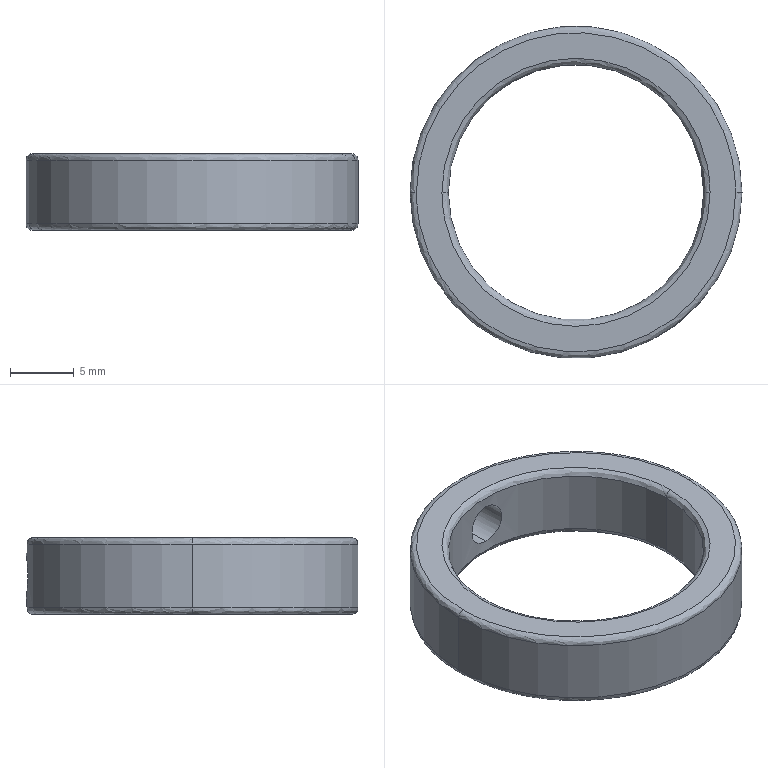Part | STEP file | Wrench hook | 1 solid | 16 faces | box 26 x 26 x 6 mm | volume 1260 mm3 | spline 8 | cylinder 6 | plane 2 | commonest cylinder face diameters 3.3 x2 20 x2 26 x2